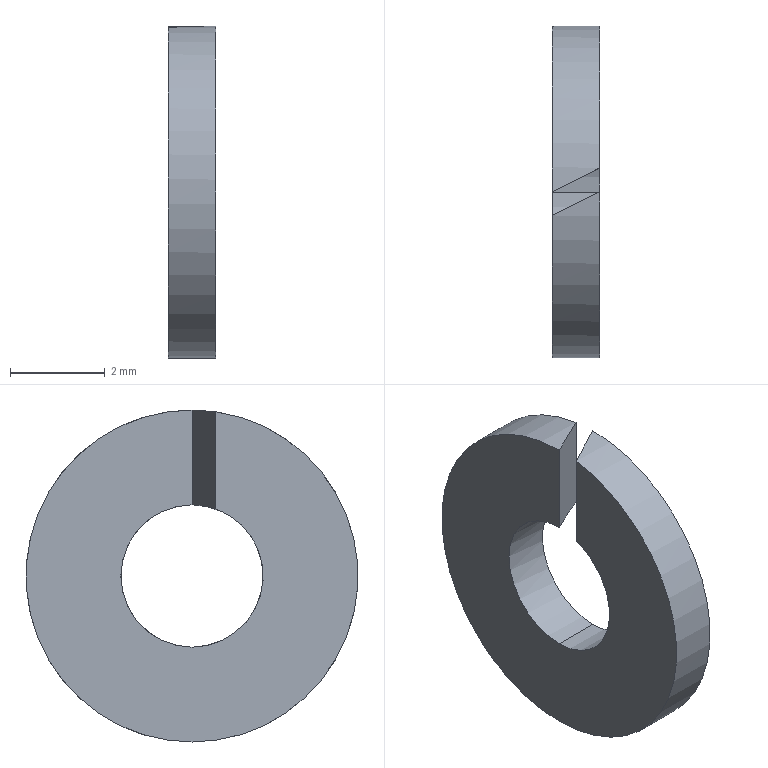Part | STEP file | 0243_Z_SCBZ4-8_2 | 1 solid | 8 faces | box 1 x 7 x 7 mm | volume 30.412 mm3 | cylinder 4 | plane 4 | commonest cylinder face diameters 3 x2 7 x2
STEP:
#1=CARTESIAN_POINT('',(0.,0.,0.));
#2=DIRECTION('',(0.,0.,1.));
#3=DIRECTION('',(1.,0.,0.));
#4=AXIS2_PLACEMENT_3D('',#1,#2,#3);
#5=CARTESIAN_POINT('',(0.,0.,-3.5));
#6=VERTEX_POINT('',#5);
#7=CARTESIAN_POINT('',(0.,-0.5,3.464));
#8=VERTEX_POINT('',#7);
#9=CARTESIAN_POINT('',(0.,0.,0.));
#10=DIRECTION('',(-1.,0.,0.));
#11=DIRECTION('',(0.,0.,-1.));
#12=AXIS2_PLACEMENT_3D('',#9,#10,#11);
#13=CIRCLE('',#12,3.5);
#14=CARTESIAN_POINT('',(0.5,0.,0.));
#15=DIRECTION('',(1.,0.,0.));
#16=DIRECTION('',(0.,0.,-1.));
#17=AXIS2_PLACEMENT_3D('',#14,#15,#16);
#18=CYLINDRICAL_SURFACE('',#17,3.5);
#19=CARTESIAN_POINT('',(6.283,-0.5));
#20=DIRECTION('',(-1.,0.));
#21=VECTOR('',#20,1.);
#22=LINE('',#19,#21);
#23=(GEOMETRIC_REPRESENTATION_CONTEXT(2)PARAMETRIC_REPRESENTATION_CONTEXT()REPRESENTATION_CONTEXT('',''));
#24=DEFINITIONAL_REPRESENTATION('',(#22),#23);
#25=PCURVE('',#18,#24);
#26=CARTESIAN_POINT('',(0.,2.5,0.));
#27=DIRECTION('',(-1.,0.,0.));
#28=DIRECTION('',(0.,0.,1.));
#29=AXIS2_PLACEMENT_3D('',#26,#27,#28);
#30=PLANE('',#29);
#31=CARTESIAN_POINT('',(0.,-2.5));
#32=DIRECTION('',(-1.,0.));
#33=AXIS2_PLACEMENT_2D('',#31,#32);
#34=CIRCLE('',#33,3.5);
#35=(GEOMETRIC_REPRESENTATION_CONTEXT(2)PARAMETRIC_REPRESENTATION_CONTEXT()REPRESENTATION_CONTEXT('',''));
#36=DEFINITIONAL_REPRESENTATION('',(#34),#35);
#37=PCURVE('',#30,#36);
#38=SURFACE_CURVE('',#13,(#25,#37),.PCURVE_S1.);
#39=EDGE_CURVE('',#6,#8,#38,.T.);
#40=ORIENTED_EDGE('',*,*,#39,.F.);
#41=CARTESIAN_POINT('',(1.,0.,-3.5));
#42=VERTEX_POINT('',#41);
#43=CARTESIAN_POINT('',(0.5,0.,-3.5));
#44=DIRECTION('',(1.,0.,0.));
#45=VECTOR('',#44,1.);
#46=LINE('',#43,#45);
#47=CARTESIAN_POINT('',(6.283,0.));
#48=DIRECTION('',(0.,1.));
#49=VECTOR('',#48,1.);
#50=LINE('',#47,#49);
#51=(GEOMETRIC_REPRESENTATION_CONTEXT(2)PARAMETRIC_REPRESENTATION_CONTEXT()REPRESENTATION_CONTEXT('',''));
#52=DEFINITIONAL_REPRESENTATION('',(#50),#51);
#53=PCURVE('',#18,#52);
#54=CARTESIAN_POINT('',(0.5,0.,0.));
#55=DIRECTION('',(1.,0.,0.));
#56=DIRECTION('',(0.,0.,-1.));
#57=AXIS2_PLACEMENT_3D('',#54,#55,#56);
#58=CYLINDRICAL_SURFACE('',#57,3.5);
#59=CARTESIAN_POINT('',(0.,0.));
#60=DIRECTION('',(0.,1.));
#61=VECTOR('',#60,1.);
#62=LINE('',#59,#61);
#63=(GEOMETRIC_REPRESENTATION_CONTEXT(2)PARAMETRIC_REPRESENTATION_CONTEXT()REPRESENTATION_CONTEXT('',''));
#64=DEFINITIONAL_REPRESENTATION('',(#62),#63);
#65=PCURVE('',#58,#64);
#66=SURFACE_CURVE('',#46,(#53,#65),.PCURVE_S1.);
#67=EDGE_CURVE('',#6,#42,#66,.T.);
#68=ORIENTED_EDGE('',*,*,#67,.T.);
#69=CARTESIAN_POINT('',(1.,0.,3.5));
#70=VERTEX_POINT('',#69);
#71=CARTESIAN_POINT('',(1.,0.,0.));
#72=DIRECTION('',(-1.,0.,0.));
#73=DIRECTION('',(0.,0.,-1.));
#74=AXIS2_PLACEMENT_3D('',#71,#72,#73);
#75=CIRCLE('',#74,3.5);
#76=CARTESIAN_POINT('',(6.283,0.5));
#77=DIRECTION('',(-1.,0.));
#78=VECTOR('',#77,1.);
#79=LINE('',#76,#78);
#80=(GEOMETRIC_REPRESENTATION_CONTEXT(2)PARAMETRIC_REPRESENTATION_CONTEXT()REPRESENTATION_CONTEXT('',''));
#81=DEFINITIONAL_REPRESENTATION('',(#79),#80);
#82=PCURVE('',#18,#81);
#83=CARTESIAN_POINT('',(1.,2.5,0.));
#84=DIRECTION('',(1.,0.,0.));
#85=DIRECTION('',(0.,0.,-1.));
#86=AXIS2_PLACEMENT_3D('',#83,#84,#85);
#87=PLANE('',#86);
#88=CARTESIAN_POINT('',(3.5,-2.5));
#89=CARTESIAN_POINT('',(3.5,-8.562));
#90=CARTESIAN_POINT('',(-1.75,-5.531));
#91=CARTESIAN_POINT('',(-7.,-2.5));
#92=CARTESIAN_POINT('',(-1.75,0.5311));
#93=CARTESIAN_POINT('',(3.5,3.562));
#94=CARTESIAN_POINT('',(3.5,-2.5));
#95=(BOUNDED_CURVE()B_SPLINE_CURVE(2,(#88,#89,#90,#91,#92,#93,#94),.UNSPECIFIED.,.T.,.F.)B_SPLINE_CURVE_WITH_KNOTS((1,2,2,2,2,1),(-2.094,0.,2.094,4.189,6.283,8.378),.UNSPECIFIED.)CURVE()GEOMETRIC_REPRESENTATION_ITEM()RATIONAL_B_SPLINE_CURVE((1.,0.5,1.,0.5,1.,0.5,1.))REPRESENTATION_ITEM(''));
#96=(GEOMETRIC_REPRESENTATION_CONTEXT(2)PARAMETRIC_REPRESENTATION_CONTEXT()REPRESENTATION_CONTEXT('',''));
#97=DEFINITIONAL_REPRESENTATION('',(#95),#96);
#98=PCURVE('',#87,#97);
#99=SURFACE_CURVE('',#75,(#82,#98),.PCURVE_S1.);
#100=EDGE_CURVE('',#42,#70,#99,.T.);
#101=ORIENTED_EDGE('',*,*,#100,.T.);
#102=CARTESIAN_POINT('',(1.,0.,3.5));
#103=CARTESIAN_POINT('',(0.6652,-0.1674,3.5));
#104=CARTESIAN_POINT('',(0.3313,-0.3343,3.488));
#105=CARTESIAN_POINT('',(0.,-0.5,3.464));
#106=(BOUNDED_CURVE()B_SPLINE_CURVE(3,(#102,#103,#104,#105),.UNSPECIFIED.,.F.,.F.)B_SPLINE_CURVE_WITH_KNOTS((4,4),(1.571,1.714),.PIECEWISE_BEZIER_KNOTS.)CURVE()GEOMETRIC_REPRESENTATION_ITEM()RATIONAL_B_SPLINE_CURVE((1.,0.9983,0.9983,1.))REPRESENTATION_ITEM(''));
#107=CARTESIAN_POINT('',(3.142,0.5));
#108=CARTESIAN_POINT('',(3.144,0.4848));
#109=CARTESIAN_POINT('',(3.148,0.4544));
#110=CARTESIAN_POINT('',(3.155,0.4088));
#111=CARTESIAN_POINT('',(3.161,0.3633));
#112=CARTESIAN_POINT('',(3.168,0.3177));
#113=CARTESIAN_POINT('',(3.174,0.2721));
#114=CARTESIAN_POINT('',(3.181,0.2265));
#115=CARTESIAN_POINT('',(3.187,0.1809));
#116=CARTESIAN_POINT('',(3.194,0.1353));
#117=CARTESIAN_POINT('',(3.2,0.08978));
#118=CARTESIAN_POINT('',(3.207,0.04423));
#119=CARTESIAN_POINT('',(3.213,-0.001291));
#120=CARTESIAN_POINT('',(3.22,-0.04679));
#121=CARTESIAN_POINT('',(3.226,-0.09227));
#122=CARTESIAN_POINT('',(3.233,-0.1377));
#123=CARTESIAN_POINT('',(3.239,-0.1831));
#124=CARTESIAN_POINT('',(3.246,-0.2285));
#125=CARTESIAN_POINT('',(3.252,-0.2739));
#126=CARTESIAN_POINT('',(3.259,-0.3192));
#127=CARTESIAN_POINT('',(3.265,-0.3645));
#128=CARTESIAN_POINT('',(3.272,-0.4097));
#129=CARTESIAN_POINT('',(3.278,-0.4549));
#130=CARTESIAN_POINT('',(3.283,-0.485));
#131=CARTESIAN_POINT('',(3.285,-0.5));
#132=B_SPLINE_CURVE_WITH_KNOTS('',3,(#107,#108,#109,#110,#111,#112,#113,#114,#115,#116,#117,#118,#119,#120,#121,#122,#123,#124,#125,#126,#127,#128,#129,#130,#131),.UNSPECIFIED.,.F.,.F.,(4,1,1,1,1,1,1,1,1,1,1,1,1,1,1,1,1,1,1,1,1,1,4),(1.571,1.577,1.584,1.59,1.597,1.603,1.61,1.616,1.623,1.629,1.636,1.642,1.649,1.656,1.662,1.669,1.675,1.682,1.688,1.695,1.701,1.708,1.714),.QUASI_UNIFORM_KNOTS.);
#133=(GEOMETRIC_REPRESENTATION_CONTEXT(2)PARAMETRIC_REPRESENTATION_CONTEXT()REPRESENTATION_CONTEXT('',''));
#134=DEFINITIONAL_REPRESENTATION('',(#132),#133);
#135=PCURVE('',#18,#134);
#136=CARTESIAN_POINT('',(1.,0.,0.));
#137=DIRECTION('',(0.4472,-0.8944,0.));
#138=DIRECTION('',(0.8944,0.4472,0.));
#139=AXIS2_PLACEMENT_3D('',#136,#137,#138);
#140=PLANE('',#139);
#141=CARTESIAN_POINT('',(0.,3.5));
#142=CARTESIAN_POINT('',(-0.3743,3.5));
#143=CARTESIAN_POINT('',(-0.7476,3.488));
#144=CARTESIAN_POINT('',(-1.118,3.464));
#145=(BOUNDED_CURVE()B_SPLINE_CURVE(3,(#141,#142,#143,#144),.UNSPECIFIED.,.F.,.F.)B_SPLINE_CURVE_WITH_KNOTS((4,4),(1.571,1.714),.PIECEWISE_BEZIER_KNOTS.)CURVE()GEOMETRIC_REPRESENTATION_ITEM()RATIONAL_B_SPLINE_CURVE((1.,0.9983,0.9983,1.))REPRESENTATION_ITEM(''));
#146=(GEOMETRIC_REPRESENTATION_CONTEXT(2)PARAMETRIC_REPRESENTATION_CONTEXT()REPRESENTATION_CONTEXT('',''));
#147=DEFINITIONAL_REPRESENTATION('',(#145),#146);
#148=PCURVE('',#140,#147);
#149=SURFACE_CURVE('',#106,(#135,#148),.PCURVE_S1.);
#150=EDGE_CURVE('',#70,#8,#149,.T.);
#151=ORIENTED_EDGE('',*,*,#150,.T.);
#152=EDGE_LOOP('',(#40,#68,#101,#151));
#153=FACE_BOUND('',#152,.T.);
#154=ADVANCED_FACE('',(#153),#18,.T.);
#155=CARTESIAN_POINT('',(1.,0.5,1.414));
#156=VERTEX_POINT('',#155);
#157=CARTESIAN_POINT('',(0.,0.,1.5));
#158=VERTEX_POINT('',#157);
#159=CARTESIAN_POINT('',(1.,0.5,1.414));
#160=CARTESIAN_POINT('',(0.678,0.339,1.471));
#161=CARTESIAN_POINT('',(0.3415,0.1707,1.5));
#162=CARTESIAN_POINT('',(0.,0.,1.5));
#163=(BOUNDED_CURVE()B_SPLINE_CURVE(3,(#159,#160,#161,#162),.UNSPECIFIED.,.F.,.F.)B_SPLINE_CURVE_WITH_KNOTS((4,4),(1.231,1.571),.PIECEWISE_BEZIER_KNOTS.)CURVE()GEOMETRIC_REPRESENTATION_ITEM()RATIONAL_B_SPLINE_CURVE((1.,0.9904,0.9904,1.))REPRESENTATION_ITEM(''));
#164=CARTESIAN_POINT('',(0.5,0.,0.));
#165=DIRECTION('',(1.,0.,0.));
#166=DIRECTION('',(0.,0.,-1.));
#167=AXIS2_PLACEMENT_3D('',#164,#165,#166);
#168=CYLINDRICAL_SURFACE('',#167,1.5);
#169=CARTESIAN_POINT('',(2.802,0.5));
#170=CARTESIAN_POINT('',(2.807,0.4855));
#171=CARTESIAN_POINT('',(2.817,0.4564));
#172=CARTESIAN_POINT('',(2.833,0.4125));
#173=CARTESIAN_POINT('',(2.848,0.3683));
#174=CARTESIAN_POINT('',(2.863,0.3239));
#175=CARTESIAN_POINT('',(2.879,0.2793));
#176=CARTESIAN_POINT('',(2.894,0.2344));
#177=CARTESIAN_POINT('',(2.91,0.1893));
#178=CARTESIAN_POINT('',(2.925,0.1441));
#179=CARTESIAN_POINT('',(2.941,0.09863));
#180=CARTESIAN_POINT('',(2.956,0.05305));
#181=CARTESIAN_POINT('',(2.972,0.007326));
#182=CARTESIAN_POINT('',(2.987,-0.03852));
#183=CARTESIAN_POINT('',(3.003,-0.08447));
#184=CARTESIAN_POINT('',(3.018,-0.1305));
#185=CARTESIAN_POINT('',(3.034,-0.1766));
#186=CARTESIAN_POINT('',(3.049,-0.2228));
#187=CARTESIAN_POINT('',(3.065,-0.269));
#188=CARTESIAN_POINT('',(3.08,-0.3152));
#189=CARTESIAN_POINT('',(3.095,-0.3614));
#190=CARTESIAN_POINT('',(3.111,-0.4077));
#191=CARTESIAN_POINT('',(3.126,-0.4539));
#192=CARTESIAN_POINT('',(3.136,-0.4846));
#193=CARTESIAN_POINT('',(3.142,-0.5));
#194=B_SPLINE_CURVE_WITH_KNOTS('',3,(#169,#170,#171,#172,#173,#174,#175,#176,#177,#178,#179,#180,#181,#182,#183,#184,#185,#186,#187,#188,#189,#190,#191,#192,#193),.UNSPECIFIED.,.F.,.F.,(4,1,1,1,1,1,1,1,1,1,1,1,1,1,1,1,1,1,1,1,1,1,4),(1.231,1.246,1.262,1.277,1.293,1.308,1.324,1.339,1.355,1.37,1.385,1.401,1.416,1.432,1.447,1.463,1.478,1.494,1.509,1.524,1.54,1.555,1.571),.QUASI_UNIFORM_KNOTS.);
#195=(GEOMETRIC_REPRESENTATION_CONTEXT(2)PARAMETRIC_REPRESENTATION_CONTEXT()REPRESENTATION_CONTEXT('',''));
#196=DEFINITIONAL_REPRESENTATION('',(#194),#195);
#197=PCURVE('',#168,#196);
#198=CARTESIAN_POINT('',(0.,0.,0.));
#199=DIRECTION('',(-0.4472,0.8944,0.));
#200=DIRECTION('',(-0.8944,-0.4472,0.));
#201=AXIS2_PLACEMENT_3D('',#198,#199,#200);
#202=PLANE('',#201);
#203=CARTESIAN_POINT('',(-1.118,1.414));
#204=CARTESIAN_POINT('',(-0.7581,1.471));
#205=CARTESIAN_POINT('',(-0.3818,1.5));
#206=CARTESIAN_POINT('',(0.,1.5));
#207=(BOUNDED_CURVE()B_SPLINE_CURVE(3,(#203,#204,#205,#206),.UNSPECIFIED.,.F.,.F.)B_SPLINE_CURVE_WITH_KNOTS((4,4),(1.231,1.571),.PIECEWISE_BEZIER_KNOTS.)CURVE()GEOMETRIC_REPRESENTATION_ITEM()RATIONAL_B_SPLINE_CURVE((1.,0.9904,0.9904,1.))REPRESENTATION_ITEM(''));
#208=(GEOMETRIC_REPRESENTATION_CONTEXT(2)PARAMETRIC_REPRESENTATION_CONTEXT()REPRESENTATION_CONTEXT('',''));
#209=DEFINITIONAL_REPRESENTATION('',(#207),#208);
#210=PCURVE('',#202,#209);
#211=SURFACE_CURVE('',#163,(#197,#210),.PCURVE_S1.);
#212=EDGE_CURVE('',#156,#158,#211,.T.);
#213=ORIENTED_EDGE('',*,*,#212,.F.);
#214=CARTESIAN_POINT('',(1.,0.,-1.5));
#215=VERTEX_POINT('',#214);
#216=CARTESIAN_POINT('',(1.,0.,0.));
#217=DIRECTION('',(-1.,0.,0.));
#218=DIRECTION('',(0.,0.,-1.));
#219=AXIS2_PLACEMENT_3D('',#216,#217,#218);
#220=CIRCLE('',#219,1.5);
#221=CARTESIAN_POINT('',(6.283,0.5));
#222=DIRECTION('',(-1.,0.));
#223=VECTOR('',#222,1.);
#224=LINE('',#221,#223);
#225=(GEOMETRIC_REPRESENTATION_CONTEXT(2)PARAMETRIC_REPRESENTATION_CONTEXT()REPRESENTATION_CONTEXT('',''));
#226=DEFINITIONAL_REPRESENTATION('',(#224),#225);
#227=PCURVE('',#168,#226);
#228=CARTESIAN_POINT('',(1.5,-2.5));
#229=CARTESIAN_POINT('',(1.5,-5.098));
#230=CARTESIAN_POINT('',(-0.75,-3.799));
#231=CARTESIAN_POINT('',(-3.,-2.5));
#232=CARTESIAN_POINT('',(-0.75,-1.201));
#233=CARTESIAN_POINT('',(1.5,0.09808));
#234=CARTESIAN_POINT('',(1.5,-2.5));
#235=(BOUNDED_CURVE()B_SPLINE_CURVE(2,(#228,#229,#230,#231,#232,#233,#234),.UNSPECIFIED.,.T.,.F.)B_SPLINE_CURVE_WITH_KNOTS((1,2,2,2,2,1),(-2.094,0.,2.094,4.189,6.283,8.378),.UNSPECIFIED.)CURVE()GEOMETRIC_REPRESENTATION_ITEM()RATIONAL_B_SPLINE_CURVE((1.,0.5,1.,0.5,1.,0.5,1.))REPRESENTATION_ITEM(''));
#236=(GEOMETRIC_REPRESENTATION_CONTEXT(2)PARAMETRIC_REPRESENTATION_CONTEXT()REPRESENTATION_CONTEXT('',''));
#237=DEFINITIONAL_REPRESENTATION('',(#235),#236);
#238=PCURVE('',#87,#237);
#239=SURFACE_CURVE('',#220,(#227,#238),.PCURVE_S1.);
#240=EDGE_CURVE('',#156,#215,#239,.T.);
#241=ORIENTED_EDGE('',*,*,#240,.T.);
#242=CARTESIAN_POINT('',(0.,0.,-1.5));
#243=VERTEX_POINT('',#242);
#244=CARTESIAN_POINT('',(0.5,0.,-1.5));
#245=DIRECTION('',(1.,0.,0.));
#246=VECTOR('',#245,1.);
#247=LINE('',#244,#246);
#248=CARTESIAN_POINT('',(0.,0.));
#249=DIRECTION('',(0.,1.));
#250=VECTOR('',#249,1.);
#251=LINE('',#248,#250);
#252=(GEOMETRIC_REPRESENTATION_CONTEXT(2)PARAMETRIC_REPRESENTATION_CONTEXT()REPRESENTATION_CONTEXT('',''));
#253=DEFINITIONAL_REPRESENTATION('',(#251),#252);
#254=PCURVE('',#168,#253);
#255=CARTESIAN_POINT('',(0.5,0.,0.));
#256=DIRECTION('',(1.,0.,0.));
#257=DIRECTION('',(0.,0.,-1.));
#258=AXIS2_PLACEMENT_3D('',#255,#256,#257);
#259=CYLINDRICAL_SURFACE('',#258,1.5);
#260=CARTESIAN_POINT('',(6.283,0.));
#261=DIRECTION('',(0.,1.));
#262=VECTOR('',#261,1.);
#263=LINE('',#260,#262);
#264=(GEOMETRIC_REPRESENTATION_CONTEXT(2)PARAMETRIC_REPRESENTATION_CONTEXT()REPRESENTATION_CONTEXT('',''));
#265=DEFINITIONAL_REPRESENTATION('',(#263),#264);
#266=PCURVE('',#259,#265);
#267=SURFACE_CURVE('',#247,(#254,#266),.PCURVE_S1.);
#268=EDGE_CURVE('',#243,#215,#267,.T.);
#269=ORIENTED_EDGE('',*,*,#268,.F.);
#270=CARTESIAN_POINT('',(0.,0.,0.));
#271=DIRECTION('',(1.,0.,0.));
#272=DIRECTION('',(0.,0.,-1.));
#273=AXIS2_PLACEMENT_3D('',#270,#271,#272);
#274=CIRCLE('',#273,1.5);
#275=CARTESIAN_POINT('',(0.,-0.5));
#276=DIRECTION('',(1.,0.));
#277=VECTOR('',#276,1.);
#278=LINE('',#275,#277);
#279=(GEOMETRIC_REPRESENTATION_CONTEXT(2)PARAMETRIC_REPRESENTATION_CONTEXT()REPRESENTATION_CONTEXT('',''));
#280=DEFINITIONAL_REPRESENTATION('',(#278),#279);
#281=PCURVE('',#168,#280);
#282=CARTESIAN_POINT('',(-1.5,-2.5));
#283=CARTESIAN_POINT('',(-1.5,0.09808));
#284=CARTESIAN_POINT('',(0.75,-1.201));
#285=CARTESIAN_POINT('',(3.,-2.5));
#286=CARTESIAN_POINT('',(0.75,-3.799));
#287=CARTESIAN_POINT('',(-1.5,-5.098));
#288=CARTESIAN_POINT('',(-1.5,-2.5));
#289=(BOUNDED_CURVE()B_SPLINE_CURVE(2,(#282,#283,#284,#285,#286,#287,#288),.UNSPECIFIED.,.T.,.F.)B_SPLINE_CURVE_WITH_KNOTS((1,2,2,2,2,1),(-2.094,0.,2.094,4.189,6.283,8.378),.UNSPECIFIED.)CURVE()GEOMETRIC_REPRESENTATION_ITEM()RATIONAL_B_SPLINE_CURVE((1.,0.5,1.,0.5,1.,0.5,1.))REPRESENTATION_ITEM(''));
#290=(GEOMETRIC_REPRESENTATION_CONTEXT(2)PARAMETRIC_REPRESENTATION_CONTEXT()REPRESENTATION_CONTEXT('',''));
#291=DEFINITIONAL_REPRESENTATION('',(#289),#290);
#292=PCURVE('',#30,#291);
#293=SURFACE_CURVE('',#274,(#281,#292),.PCURVE_S1.);
#294=EDGE_CURVE('',#243,#158,#293,.T.);
#295=ORIENTED_EDGE('',*,*,#294,.T.);
#296=EDGE_LOOP('',(#213,#241,#269,#295));
#297=FACE_BOUND('',#296,.F.);
#298=ADVANCED_FACE('',(#297),#168,.F.);
#299=CARTESIAN_POINT('',(0.,0.,3.5));
#300=VERTEX_POINT('',#299);
#301=CARTESIAN_POINT('',(0.,0.,0.));
#302=DIRECTION('',(-1.,0.,0.));
#303=DIRECTION('',(0.,0.,-1.));
#304=AXIS2_PLACEMENT_3D('',#301,#302,#303);
#305=CIRCLE('',#304,3.5);
#306=CARTESIAN_POINT('',(0.,-2.5));
#307=DIRECTION('',(-1.,0.));
#308=AXIS2_PLACEMENT_2D('',#306,#307);
#309=CIRCLE('',#308,3.5);
#310=(GEOMETRIC_REPRESENTATION_CONTEXT(2)PARAMETRIC_REPRESENTATION_CONTEXT()REPRESENTATION_CONTEXT('',''));
#311=DEFINITIONAL_REPRESENTATION('',(#309),#310);
#312=PCURVE('',#30,#311);
#313=CARTESIAN_POINT('',(6.283,-0.5));
#314=DIRECTION('',(-1.,0.));
#315=VECTOR('',#314,1.);
#316=LINE('',#313,#315);
#317=(GEOMETRIC_REPRESENTATION_CONTEXT(2)PARAMETRIC_REPRESENTATION_CONTEXT()REPRESENTATION_CONTEXT('',''));
#318=DEFINITIONAL_REPRESENTATION('',(#316),#317);
#319=PCURVE('',#58,#318);
#320=SURFACE_CURVE('',#305,(#312,#319),.PCURVE_S1.);
#321=EDGE_CURVE('',#300,#6,#320,.T.);
#322=ORIENTED_EDGE('',*,*,#321,.T.);
#323=ORIENTED_EDGE('',*,*,#39,.T.);
#324=CARTESIAN_POINT('',(0.,-0.5,1.414));
#325=VERTEX_POINT('',#324);
#326=CARTESIAN_POINT('',(0.,-0.5,0.));
#327=DIRECTION('',(0.,0.,-1.));
#328=VECTOR('',#327,1.);
#329=LINE('',#326,#328);
#330=CARTESIAN_POINT('',(0.,-3.));
#331=DIRECTION('',(-1.,0.));
#332=VECTOR('',#331,1.);
#333=LINE('',#330,#332);
#334=(GEOMETRIC_REPRESENTATION_CONTEXT(2)PARAMETRIC_REPRESENTATION_CONTEXT()REPRESENTATION_CONTEXT('',''));
#335=DEFINITIONAL_REPRESENTATION('',(#333),#334);
#336=PCURVE('',#30,#335);
#337=CARTESIAN_POINT('',(-1.118,0.));
#338=DIRECTION('',(0.,-1.));
#339=VECTOR('',#338,1.);
#340=LINE('',#337,#339);
#341=(GEOMETRIC_REPRESENTATION_CONTEXT(2)PARAMETRIC_REPRESENTATION_CONTEXT()REPRESENTATION_CONTEXT('',''));
#342=DEFINITIONAL_REPRESENTATION('',(#340),#341);
#343=PCURVE('',#140,#342);
#344=SURFACE_CURVE('',#329,(#336,#343),.PCURVE_S1.);
#345=EDGE_CURVE('',#8,#325,#344,.T.);
#346=ORIENTED_EDGE('',*,*,#345,.T.);
#347=CARTESIAN_POINT('',(0.,0.,0.));
#348=DIRECTION('',(1.,0.,0.));
#349=DIRECTION('',(0.,0.,-1.));
#350=AXIS2_PLACEMENT_3D('',#347,#348,#349);
#351=CIRCLE('',#350,1.5);
#352=CARTESIAN_POINT('',(-1.5,-2.5));
#353=CARTESIAN_POINT('',(-1.5,0.09808));
#354=CARTESIAN_POINT('',(0.75,-1.201));
#355=CARTESIAN_POINT('',(3.,-2.5));
#356=CARTESIAN_POINT('',(0.75,-3.799));
#357=CARTESIAN_POINT('',(-1.5,-5.098));
#358=CARTESIAN_POINT('',(-1.5,-2.5));
#359=(BOUNDED_CURVE()B_SPLINE_CURVE(2,(#352,#353,#354,#355,#356,#357,#358),.UNSPECIFIED.,.T.,.F.)B_SPLINE_CURVE_WITH_KNOTS((1,2,2,2,2,1),(-2.094,0.,2.094,4.189,6.283,8.378),.UNSPECIFIED.)CURVE()GEOMETRIC_REPRESENTATION_ITEM()RATIONAL_B_SPLINE_CURVE((1.,0.5,1.,0.5,1.,0.5,1.))REPRESENTATION_ITEM(''));
#360=(GEOMETRIC_REPRESENTATION_CONTEXT(2)PARAMETRIC_REPRESENTATION_CONTEXT()REPRESENTATION_CONTEXT('',''));
#361=DEFINITIONAL_REPRESENTATION('',(#359),#360);
#362=PCURVE('',#30,#361);
#363=CARTESIAN_POINT('',(0.,-0.5));
#364=DIRECTION('',(1.,0.));
#365=VECTOR('',#364,1.);
#366=LINE('',#363,#365);
#367=(GEOMETRIC_REPRESENTATION_CONTEXT(2)PARAMETRIC_REPRESENTATION_CONTEXT()REPRESENTATION_CONTEXT('',''));
#368=DEFINITIONAL_REPRESENTATION('',(#366),#367);
#369=PCURVE('',#259,#368);
#370=SURFACE_CURVE('',#351,(#362,#369),.PCURVE_S1.);
#371=EDGE_CURVE('',#325,#243,#370,.T.);
#372=ORIENTED_EDGE('',*,*,#371,.T.);
#373=ORIENTED_EDGE('',*,*,#294,.T.);
#374=CARTESIAN_POINT('',(0.,0.,0.));
#375=DIRECTION('',(0.,0.,1.));
#376=VECTOR('',#375,1.);
#377=LINE('',#374,#376);
#378=CARTESIAN_POINT('',(0.,-2.5));
#379=DIRECTION('',(1.,0.));
#380=VECTOR('',#379,1.);
#381=LINE('',#378,#380);
#382=(GEOMETRIC_REPRESENTATION_CONTEXT(2)PARAMETRIC_REPRESENTATION_CONTEXT()REPRESENTATION_CONTEXT('',''));
#383=DEFINITIONAL_REPRESENTATION('',(#381),#382);
#384=PCURVE('',#30,#383);
#385=CARTESIAN_POINT('',(0.,0.));
#386=DIRECTION('',(0.,1.));
#387=VECTOR('',#386,1.);
#388=LINE('',#385,#387);
#389=(GEOMETRIC_REPRESENTATION_CONTEXT(2)PARAMETRIC_REPRESENTATION_CONTEXT()REPRESENTATION_CONTEXT('',''));
#390=DEFINITIONAL_REPRESENTATION('',(#388),#389);
#391=PCURVE('',#202,#390);
#392=SURFACE_CURVE('',#377,(#384,#391),.PCURVE_S1.);
#393=EDGE_CURVE('',#158,#300,#392,.T.);
#394=ORIENTED_EDGE('',*,*,#393,.T.);
#395=EDGE_LOOP('',(#322,#323,#346,#372,#373,#394));
#396=FACE_BOUND('',#395,.T.);
#397=ADVANCED_FACE('',(#396),#30,.T.);
#398=ORIENTED_EDGE('',*,*,#67,.F.);
#399=ORIENTED_EDGE('',*,*,#321,.F.);
#400=CARTESIAN_POINT('',(1.,0.5,3.464));
#401=VERTEX_POINT('',#400);
#402=CARTESIAN_POINT('',(0.,0.,3.5));
#403=CARTESIAN_POINT('',(0.3348,0.1674,3.5));
#404=CARTESIAN_POINT('',(0.6687,0.3343,3.488));
#405=CARTESIAN_POINT('',(1.,0.5,3.464));
#406=(BOUNDED_CURVE()B_SPLINE_CURVE(3,(#402,#403,#404,#405),.UNSPECIFIED.,.F.,.F.)B_SPLINE_CURVE_WITH_KNOTS((4,4),(4.712,4.856),.PIECEWISE_BEZIER_KNOTS.)CURVE()GEOMETRIC_REPRESENTATION_ITEM()RATIONAL_B_SPLINE_CURVE((1.,0.9983,0.9983,1.))REPRESENTATION_ITEM(''));
#407=CARTESIAN_POINT('',(3.142,-0.5));
#408=CARTESIAN_POINT('',(3.139,-0.4848));
#409=CARTESIAN_POINT('',(3.135,-0.4544));
#410=CARTESIAN_POINT('',(3.129,-0.4088));
#411=CARTESIAN_POINT('',(3.122,-0.3633));
#412=CARTESIAN_POINT('',(3.116,-0.3177));
#413=CARTESIAN_POINT('',(3.109,-0.2721));
#414=CARTESIAN_POINT('',(3.103,-0.2265));
#415=CARTESIAN_POINT('',(3.096,-0.1809));
#416=CARTESIAN_POINT('',(3.089,-0.1353));
#417=CARTESIAN_POINT('',(3.083,-0.08978));
#418=CARTESIAN_POINT('',(3.076,-0.04423));
#419=CARTESIAN_POINT('',(3.07,0.001291));
#420=CARTESIAN_POINT('',(3.063,0.04679));
#421=CARTESIAN_POINT('',(3.057,0.09227));
#422=CARTESIAN_POINT('',(3.05,0.1377));
#423=CARTESIAN_POINT('',(3.044,0.1831));
#424=CARTESIAN_POINT('',(3.037,0.2285));
#425=CARTESIAN_POINT('',(3.031,0.2739));
#426=CARTESIAN_POINT('',(3.024,0.3192));
#427=CARTESIAN_POINT('',(3.018,0.3645));
#428=CARTESIAN_POINT('',(3.011,0.4097));
#429=CARTESIAN_POINT('',(3.005,0.4549));
#430=CARTESIAN_POINT('',(3.,0.485));
#431=CARTESIAN_POINT('',(2.998,0.5));
#432=B_SPLINE_CURVE_WITH_KNOTS('',3,(#407,#408,#409,#410,#411,#412,#413,#414,#415,#416,#417,#418,#419,#420,#421,#422,#423,#424,#425,#426,#427,#428,#429,#430,#431),.UNSPECIFIED.,.F.,.F.,(4,1,1,1,1,1,1,1,1,1,1,1,1,1,1,1,1,1,1,1,1,1,4),(4.712,4.719,4.725,4.732,4.738,4.745,4.751,4.758,4.765,4.771,4.778,4.784,4.791,4.797,4.804,4.81,4.817,4.823,4.83,4.836,4.843,4.849,4.856),.QUASI_UNIFORM_KNOTS.);
#433=(GEOMETRIC_REPRESENTATION_CONTEXT(2)PARAMETRIC_REPRESENTATION_CONTEXT()REPRESENTATION_CONTEXT('',''));
#434=DEFINITIONAL_REPRESENTATION('',(#432),#433);
#435=PCURVE('',#58,#434);
#436=CARTESIAN_POINT('',(0.,3.5));
#437=CARTESIAN_POINT('',(-0.3743,3.5));
#438=CARTESIAN_POINT('',(-0.7476,3.488));
#439=CARTESIAN_POINT('',(-1.118,3.464));
#440=(BOUNDED_CURVE()B_SPLINE_CURVE(3,(#436,#437,#438,#439),.UNSPECIFIED.,.F.,.F.)B_SPLINE_CURVE_WITH_KNOTS((4,4),(4.712,4.856),.PIECEWISE_BEZIER_KNOTS.)CURVE()GEOMETRIC_REPRESENTATION_ITEM()RATIONAL_B_SPLINE_CURVE((1.,0.9983,0.9983,1.))REPRESENTATION_ITEM(''));
#441=(GEOMETRIC_REPRESENTATION_CONTEXT(2)PARAMETRIC_REPRESENTATION_CONTEXT()REPRESENTATION_CONTEXT('',''));
#442=DEFINITIONAL_REPRESENTATION('',(#440),#441);
#443=PCURVE('',#202,#442);
#444=SURFACE_CURVE('',#406,(#435,#443),.PCURVE_S1.);
#445=EDGE_CURVE('',#300,#401,#444,.T.);
#446=ORIENTED_EDGE('',*,*,#445,.T.);
#447=CARTESIAN_POINT('',(1.,0.,0.));
#448=DIRECTION('',(-1.,0.,0.));
#449=DIRECTION('',(0.,0.,-1.));
#450=AXIS2_PLACEMENT_3D('',#447,#448,#449);
#451=CIRCLE('',#450,3.5);
#452=CARTESIAN_POINT('',(6.283,0.5));
#453=DIRECTION('',(-1.,0.));
#454=VECTOR('',#453,1.);
#455=LINE('',#452,#454);
#456=(GEOMETRIC_REPRESENTATION_CONTEXT(2)PARAMETRIC_REPRESENTATION_CONTEXT()REPRESENTATION_CONTEXT('',''));
#457=DEFINITIONAL_REPRESENTATION('',(#455),#456);
#458=PCURVE('',#58,#457);
#459=CARTESIAN_POINT('',(3.5,-2.5));
#460=CARTESIAN_POINT('',(3.5,-8.562));
#461=CARTESIAN_POINT('',(-1.75,-5.531));
#462=CARTESIAN_POINT('',(-7.,-2.5));
#463=CARTESIAN_POINT('',(-1.75,0.5311));
#464=CARTESIAN_POINT('',(3.5,3.562));
#465=CARTESIAN_POINT('',(3.5,-2.5));
#466=(BOUNDED_CURVE()B_SPLINE_CURVE(2,(#459,#460,#461,#462,#463,#464,#465),.UNSPECIFIED.,.T.,.F.)B_SPLINE_CURVE_WITH_KNOTS((1,2,2,2,2,1),(-2.094,0.,2.094,4.189,6.283,8.378),.UNSPECIFIED.)CURVE()GEOMETRIC_REPRESENTATION_ITEM()RATIONAL_B_SPLINE_CURVE((1.,0.5,1.,0.5,1.,0.5,1.))REPRESENTATION_ITEM(''));
#467=(GEOMETRIC_REPRESENTATION_CONTEXT(2)PARAMETRIC_REPRESENTATION_CONTEXT()REPRESENTATION_CONTEXT('',''));
#468=DEFINITIONAL_REPRESENTATION('',(#466),#467);
#469=PCURVE('',#87,#468);
#470=SURFACE_CURVE('',#451,(#458,#469),.PCURVE_S1.);
#471=EDGE_CURVE('',#401,#42,#470,.T.);
#472=ORIENTED_EDGE('',*,*,#471,.T.);
#473=EDGE_LOOP('',(#398,#399,#446,#472));
#474=FACE_BOUND('',#473,.T.);
#475=ADVANCED_FACE('',(#474),#58,.T.);
#476=ORIENTED_EDGE('',*,*,#393,.F.);
#477=ORIENTED_EDGE('',*,*,#212,.F.);
#478=CARTESIAN_POINT('',(1.,0.5,0.));
#479=DIRECTION('',(0.,0.,-1.));
#480=VECTOR('',#479,1.);
#481=LINE('',#478,#480);
#482=CARTESIAN_POINT('',(-1.118,0.));
#483=DIRECTION('',(0.,-1.));
#484=VECTOR('',#483,1.);
#485=LINE('',#482,#484);
#486=(GEOMETRIC_REPRESENTATION_CONTEXT(2)PARAMETRIC_REPRESENTATION_CONTEXT()REPRESENTATION_CONTEXT('',''));
#487=DEFINITIONAL_REPRESENTATION('',(#485),#486);
#488=PCURVE('',#202,#487);
#489=CARTESIAN_POINT('',(0.,-2.));
#490=DIRECTION('',(1.,0.));
#491=VECTOR('',#490,1.);
#492=LINE('',#489,#491);
#493=(GEOMETRIC_REPRESENTATION_CONTEXT(2)PARAMETRIC_REPRESENTATION_CONTEXT()REPRESENTATION_CONTEXT('',''));
#494=DEFINITIONAL_REPRESENTATION('',(#492),#493);
#495=PCURVE('',#87,#494);
#496=SURFACE_CURVE('',#481,(#488,#495),.PCURVE_S1.);
#497=EDGE_CURVE('',#401,#156,#496,.T.);
#498=ORIENTED_EDGE('',*,*,#497,.F.);
#499=ORIENTED_EDGE('',*,*,#445,.F.);
#500=EDGE_LOOP('',(#476,#477,#498,#499));
#501=FACE_BOUND('',#500,.T.);
#502=ADVANCED_FACE('',(#501),#202,.F.);
#503=CARTESIAN_POINT('',(1.,0.,1.5));
#504=VERTEX_POINT('',#503);
#505=CARTESIAN_POINT('',(1.,0.,0.));
#506=DIRECTION('',(-1.,0.,0.));
#507=DIRECTION('',(0.,0.,-1.));
#508=AXIS2_PLACEMENT_3D('',#505,#506,#507);
#509=CIRCLE('',#508,1.5);
#510=CARTESIAN_POINT('',(6.283,0.5));
#511=DIRECTION('',(-1.,0.));
#512=VECTOR('',#511,1.);
#513=LINE('',#510,#512);
#514=(GEOMETRIC_REPRESENTATION_CONTEXT(2)PARAMETRIC_REPRESENTATION_CONTEXT()REPRESENTATION_CONTEXT('',''));
#515=DEFINITIONAL_REPRESENTATION('',(#513),#514);
#516=PCURVE('',#259,#515);
#517=CARTESIAN_POINT('',(1.5,-2.5));
#518=CARTESIAN_POINT('',(1.5,-5.098));
#519=CARTESIAN_POINT('',(-0.75,-3.799));
#520=CARTESIAN_POINT('',(-3.,-2.5));
#521=CARTESIAN_POINT('',(-0.75,-1.201));
#522=CARTESIAN_POINT('',(1.5,0.09808));
#523=CARTESIAN_POINT('',(1.5,-2.5));
#524=(BOUNDED_CURVE()B_SPLINE_CURVE(2,(#517,#518,#519,#520,#521,#522,#523),.UNSPECIFIED.,.T.,.F.)B_SPLINE_CURVE_WITH_KNOTS((1,2,2,2,2,1),(-2.094,0.,2.094,4.189,6.283,8.378),.UNSPECIFIED.)CURVE()GEOMETRIC_REPRESENTATION_ITEM()RATIONAL_B_SPLINE_CURVE((1.,0.5,1.,0.5,1.,0.5,1.))REPRESENTATION_ITEM(''));
#525=(GEOMETRIC_REPRESENTATION_CONTEXT(2)PARAMETRIC_REPRESENTATION_CONTEXT()REPRESENTATION_CONTEXT('',''));
#526=DEFINITIONAL_REPRESENTATION('',(#524),#525);
#527=PCURVE('',#87,#526);
#528=SURFACE_CURVE('',#509,(#516,#527),.PCURVE_S1.);
#529=EDGE_CURVE('',#215,#504,#528,.T.);
#530=ORIENTED_EDGE('',*,*,#529,.T.);
#531=CARTESIAN_POINT('',(1.,0.,1.5));
#532=CARTESIAN_POINT('',(0.6585,-0.1707,1.5));
#533=CARTESIAN_POINT('',(0.322,-0.339,1.471));
#534=CARTESIAN_POINT('',(0.,-0.5,1.414));
#535=(BOUNDED_CURVE()B_SPLINE_CURVE(3,(#531,#532,#533,#534),.UNSPECIFIED.,.F.,.F.)B_SPLINE_CURVE_WITH_KNOTS((4,4),(1.571,1.911),.PIECEWISE_BEZIER_KNOTS.)CURVE()GEOMETRIC_REPRESENTATION_ITEM()RATIONAL_B_SPLINE_CURVE((1.,0.9904,0.9904,1.))REPRESENTATION_ITEM(''));
#536=CARTESIAN_POINT('',(3.142,0.5));
#537=CARTESIAN_POINT('',(3.147,0.4846));
#538=CARTESIAN_POINT('',(3.157,0.4539));
#539=CARTESIAN_POINT('',(3.172,0.4077));
#540=CARTESIAN_POINT('',(3.188,0.3614));
#541=CARTESIAN_POINT('',(3.203,0.3152));
#542=CARTESIAN_POINT('',(3.219,0.269));
#543=CARTESIAN_POINT('',(3.234,0.2228));
#544=CARTESIAN_POINT('',(3.25,0.1766));
#545=CARTESIAN_POINT('',(3.265,0.1305));
#546=CARTESIAN_POINT('',(3.281,0.08447));
#547=CARTESIAN_POINT('',(3.296,0.03852));
#548=CARTESIAN_POINT('',(3.312,-0.007326));
#549=CARTESIAN_POINT('',(3.327,-0.05305));
#550=CARTESIAN_POINT('',(3.342,-0.09863));
#551=CARTESIAN_POINT('',(3.358,-0.1441));
#552=CARTESIAN_POINT('',(3.373,-0.1893));
#553=CARTESIAN_POINT('',(3.389,-0.2344));
#554=CARTESIAN_POINT('',(3.404,-0.2793));
#555=CARTESIAN_POINT('',(3.42,-0.3239));
#556=CARTESIAN_POINT('',(3.435,-0.3683));
#557=CARTESIAN_POINT('',(3.451,-0.4125));
#558=CARTESIAN_POINT('',(3.466,-0.4564));
#559=CARTESIAN_POINT('',(3.476,-0.4855));
#560=CARTESIAN_POINT('',(3.481,-0.5));
#561=B_SPLINE_CURVE_WITH_KNOTS('',3,(#536,#537,#538,#539,#540,#541,#542,#543,#544,#545,#546,#547,#548,#549,#550,#551,#552,#553,#554,#555,#556,#557,#558,#559,#560),.UNSPECIFIED.,.F.,.F.,(4,1,1,1,1,1,1,1,1,1,1,1,1,1,1,1,1,1,1,1,1,1,4),(1.571,1.586,1.602,1.617,1.633,1.648,1.663,1.679,1.694,1.71,1.725,1.741,1.756,1.772,1.787,1.803,1.818,1.833,1.849,1.864,1.88,1.895,1.911),.QUASI_UNIFORM_KNOTS.);
#562=(GEOMETRIC_REPRESENTATION_CONTEXT(2)PARAMETRIC_REPRESENTATION_CONTEXT()REPRESENTATION_CONTEXT('',''));
#563=DEFINITIONAL_REPRESENTATION('',(#561),#562);
#564=PCURVE('',#259,#563);
#565=CARTESIAN_POINT('',(0.,1.5));
#566=CARTESIAN_POINT('',(-0.3818,1.5));
#567=CARTESIAN_POINT('',(-0.7581,1.471));
#568=CARTESIAN_POINT('',(-1.118,1.414));
#569=(BOUNDED_CURVE()B_SPLINE_CURVE(3,(#565,#566,#567,#568),.UNSPECIFIED.,.F.,.F.)B_SPLINE_CURVE_WITH_KNOTS((4,4),(1.571,1.911),.PIECEWISE_BEZIER_KNOTS.)CURVE()GEOMETRIC_REPRESENTATION_ITEM()RATIONAL_B_SPLINE_CURVE((1.,0.9904,0.9904,1.))REPRESENTATION_ITEM(''));
#570=(GEOMETRIC_REPRESENTATION_CONTEXT(2)PARAMETRIC_REPRESENTATION_CONTEXT()REPRESENTATION_CONTEXT('',''));
#571=DEFINITIONAL_REPRESENTATION('',(#569),#570);
#572=PCURVE('',#140,#571);
#573=SURFACE_CURVE('',#535,(#564,#572),.PCURVE_S1.);
#574=EDGE_CURVE('',#504,#325,#573,.T.);
#575=ORIENTED_EDGE('',*,*,#574,.T.);
#576=ORIENTED_EDGE('',*,*,#371,.T.);
#577=ORIENTED_EDGE('',*,*,#268,.T.);
#578=EDGE_LOOP('',(#530,#575,#576,#577));
#579=FACE_BOUND('',#578,.F.);
#580=ADVANCED_FACE('',(#579),#259,.F.);
#581=CARTESIAN_POINT('',(1.,0.,0.));
#582=DIRECTION('',(0.,0.,1.));
#583=VECTOR('',#582,1.);
#584=LINE('',#581,#583);
#585=CARTESIAN_POINT('',(0.,0.));
#586=DIRECTION('',(0.,1.));
#587=VECTOR('',#586,1.);
#588=LINE('',#585,#587);
#589=(GEOMETRIC_REPRESENTATION_CONTEXT(2)PARAMETRIC_REPRESENTATION_CONTEXT()REPRESENTATION_CONTEXT('',''));
#590=DEFINITIONAL_REPRESENTATION('',(#588),#589);
#591=PCURVE('',#140,#590);
#592=CARTESIAN_POINT('',(0.,-2.5));
#593=DIRECTION('',(-1.,0.));
#594=VECTOR('',#593,1.);
#595=LINE('',#592,#594);
#596=(GEOMETRIC_REPRESENTATION_CONTEXT(2)PARAMETRIC_REPRESENTATION_CONTEXT()REPRESENTATION_CONTEXT('',''));
#597=DEFINITIONAL_REPRESENTATION('',(#595),#596);
#598=PCURVE('',#87,#597);
#599=SURFACE_CURVE('',#584,(#591,#598),.PCURVE_S1.);
#600=EDGE_CURVE('',#504,#70,#599,.T.);
#601=ORIENTED_EDGE('',*,*,#600,.F.);
#602=ORIENTED_EDGE('',*,*,#574,.T.);
#603=ORIENTED_EDGE('',*,*,#345,.F.);
#604=ORIENTED_EDGE('',*,*,#150,.F.);
#605=EDGE_LOOP('',(#601,#602,#603,#604));
#606=FACE_BOUND('',#605,.T.);
#607=ADVANCED_FACE('',(#606),#140,.F.);
#608=ORIENTED_EDGE('',*,*,#240,.T.);
#609=ORIENTED_EDGE('',*,*,#529,.T.);
#610=ORIENTED_EDGE('',*,*,#600,.T.);
#611=ORIENTED_EDGE('',*,*,#100,.F.);
#612=ORIENTED_EDGE('',*,*,#471,.F.);
#613=ORIENTED_EDGE('',*,*,#497,.T.);
#614=EDGE_LOOP('',(#608,#609,#610,#611,#612,#613));
#615=FACE_BOUND('',#614,.T.);
#616=ADVANCED_FACE('',(#615),#87,.T.);
#617=CLOSED_SHELL('',(#154,#298,#397,#475,#502,#580,#607,#616));
#618=MANIFOLD_SOLID_BREP('',#617);
#619=(LENGTH_UNIT()NAMED_UNIT(*)SI_UNIT(.MILLI.,.METRE.));
#620=UNCERTAINTY_MEASURE_WITH_UNIT(LENGTH_MEASURE(0.0000001),#619,'','');
#621=(NAMED_UNIT(*)PLANE_ANGLE_UNIT()SI_UNIT($,.RADIAN.));
#622=(NAMED_UNIT(*)SI_UNIT($,.STERADIAN.)SOLID_ANGLE_UNIT());
#623=(GEOMETRIC_REPRESENTATION_CONTEXT(3)GLOBAL_UNCERTAINTY_ASSIGNED_CONTEXT((#620))GLOBAL_UNIT_ASSIGNED_CONTEXT((#619,#621,#622))REPRESENTATION_CONTEXT('',''));
#624=ADVANCED_BREP_SHAPE_REPRESENTATION('',(#4,#618),#623);